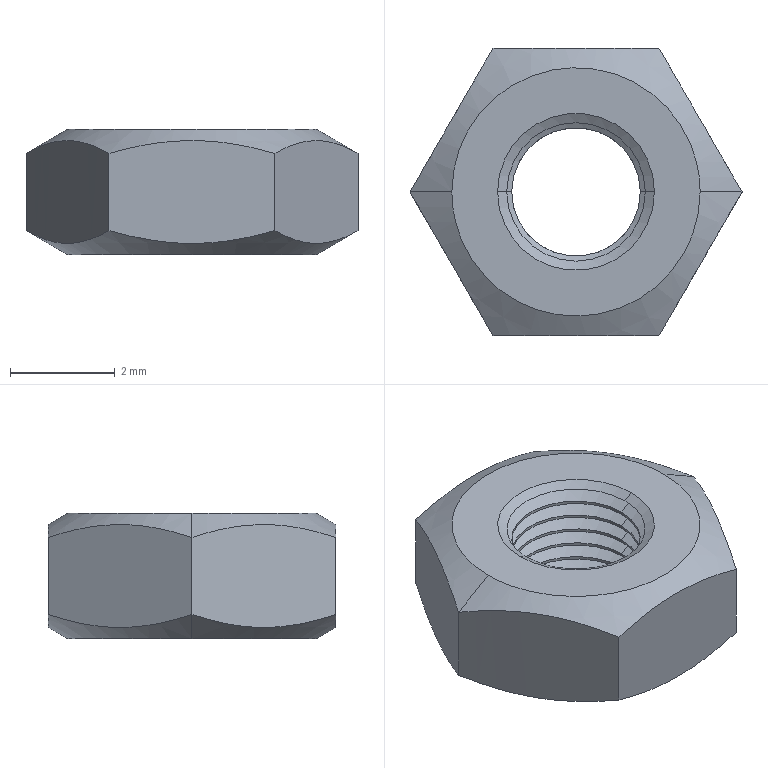Part | STEP file | PN_0012_Default<As Machined> | 1 solid | 56 faces | box 6.351 x 5.5 x 2.4 mm | volume 46.625 mm3 | cone 36 | cylinder 12 | plane 8 | commonest cylinder face diameters 2.459 x12